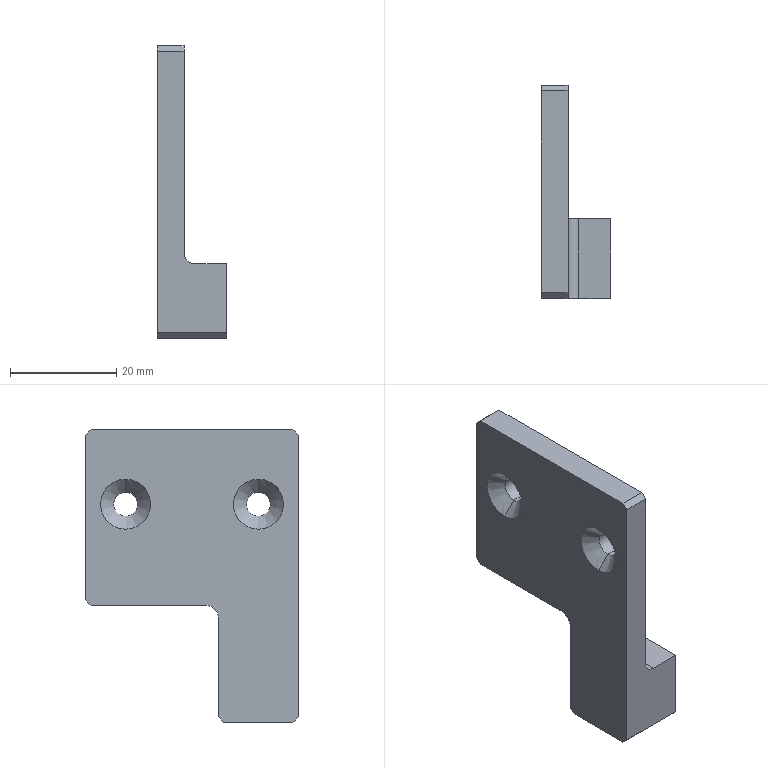Part | STEP file | 1 solid | 29 faces | box 13 x 40 x 55 mm | volume 9570 mm3 | plane 15 | cylinder 8 | cone 6 | commonest cylinder face diameters 4.5 x4 3.3 x2 4 x1 5 x1